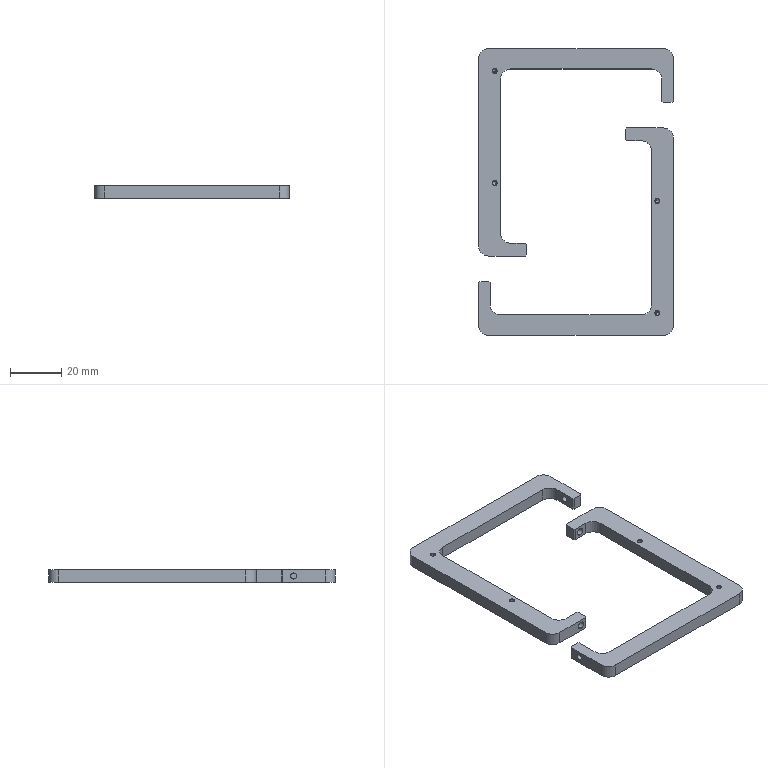Part | 2 solids | 80 faces | box 76 x 112 x 5 mm | volume 13239 mm3 | plane 32 | cylinder 28 | cone 20 | commonest cylinder face diameters 8 x12 1.6 x8 2.4 x4 2.9 x4